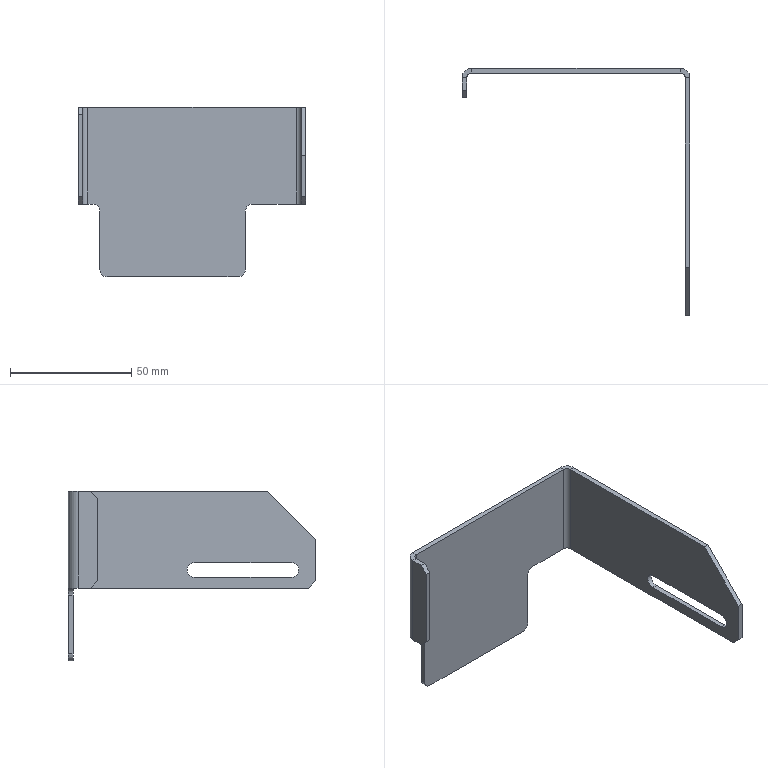Part | NX | features BREP 1 | 1 solid | 38 faces | box 94 x 102 x 70 mm | volume 18750 mm3 | plane 28 | cylinder 10 | commonest cylinder face diameters 6 x6 4 x2 8 x2
STEP:
#1=CARTESIAN_POINT('',(-43.,2.,-20.));
#2=VERTEX_POINT('',#1);
#3=CARTESIAN_POINT('',(-41.,2.,-20.));
#4=VERTEX_POINT('',#3);
#5=CARTESIAN_POINT('',(-45.,2.,-20.));
#6=DIRECTION('',(1.,0.,0.));
#7=VECTOR('',#6,1000.);
#8=LINE('',#5,#7);
#9=EDGE_CURVE('',#2,#4,#8,.T.);
#10=ORIENTED_EDGE('',*,*,#9,.T.);
#11=CARTESIAN_POINT('',(-41.,0.,-20.));
#12=VERTEX_POINT('',#11);
#13=CARTESIAN_POINT('',(-41.,-2.,-20.));
#14=DIRECTION('',(0.,-1.,0.));
#15=VECTOR('',#14,1000.);
#16=LINE('',#13,#15);
#17=EDGE_CURVE('',#4,#12,#16,.T.);
#18=ORIENTED_EDGE('',*,*,#17,.T.);
#19=CARTESIAN_POINT('',(-43.,0.,-20.));
#20=VERTEX_POINT('',#19);
#21=CARTESIAN_POINT('',(-45.,0.,-20.));
#22=DIRECTION('',(1.,0.,0.));
#23=VECTOR('',#22,1000.);
#24=LINE('',#21,#23);
#25=EDGE_CURVE('',#20,#12,#24,.T.);
#26=ORIENTED_EDGE('',*,*,#25,.F.);
#27=CARTESIAN_POINT('',(-43.,0.,-20.));
#28=DIRECTION('',(0.,1.,0.));
#29=VECTOR('',#28,1000.);
#30=LINE('',#27,#29);
#31=EDGE_CURVE('',#20,#2,#30,.T.);
#32=ORIENTED_EDGE('',*,*,#31,.T.);
#33=EDGE_LOOP('',(#10,#18,#26,#32));
#34=FACE_BOUND('',#33,.T.);
#35=CARTESIAN_POINT('',(43.,-2.,-20.));
#36=DIRECTION('',(0.,0.,1.));
#37=DIRECTION('',(-1.,0.,0.));
#38=AXIS2_PLACEMENT_3D('',#35,#36,#37);
#39=PLANE('',#38);
#40=ADVANCED_FACE('',(#34),#39,.F.);
#41=CARTESIAN_POINT('',(22.,2.,-23.));
#42=VERTEX_POINT('',#41);
#43=CARTESIAN_POINT('',(22.,2.,-47.));
#44=VERTEX_POINT('',#43);
#45=CARTESIAN_POINT('',(22.,2.,-20.));
#46=DIRECTION('',(0.,0.,-1.));
#47=VECTOR('',#46,1000.);
#48=LINE('',#45,#47);
#49=EDGE_CURVE('',#42,#44,#48,.T.);
#50=ORIENTED_EDGE('',*,*,#49,.T.);
#51=CARTESIAN_POINT('',(19.,2.,-50.));
#52=VERTEX_POINT('',#51);
#53=CARTESIAN_POINT('',(19.,2.,-47.));
#54=DIRECTION('',(0.,1.,0.));
#55=DIRECTION('',(0.,0.,1.));
#56=AXIS2_PLACEMENT_3D('',#53,#54,#55);
#57=CIRCLE('',#56,3.);
#58=EDGE_CURVE('',#44,#52,#57,.T.);
#59=ORIENTED_EDGE('',*,*,#58,.T.);
#60=CARTESIAN_POINT('',(-35.,2.,-50.));
#61=VERTEX_POINT('',#60);
#62=CARTESIAN_POINT('',(-38.,2.,-50.));
#63=DIRECTION('',(-1.,0.,0.));
#64=VECTOR('',#63,1000.);
#65=LINE('',#62,#64);
#66=EDGE_CURVE('',#52,#61,#65,.T.);
#67=ORIENTED_EDGE('',*,*,#66,.T.);
#68=CARTESIAN_POINT('',(-38.,2.,-47.));
#69=VERTEX_POINT('',#68);
#70=CARTESIAN_POINT('',(-35.,2.,-47.));
#71=DIRECTION('',(0.,1.,0.));
#72=DIRECTION('',(0.,0.,1.));
#73=AXIS2_PLACEMENT_3D('',#70,#71,#72);
#74=CIRCLE('',#73,3.);
#75=EDGE_CURVE('',#61,#69,#74,.T.);
#76=ORIENTED_EDGE('',*,*,#75,.T.);
#77=CARTESIAN_POINT('',(-38.,2.,-23.));
#78=VERTEX_POINT('',#77);
#79=CARTESIAN_POINT('',(-38.,2.,-20.));
#80=DIRECTION('',(0.,0.,1.));
#81=VECTOR('',#80,1000.);
#82=LINE('',#79,#81);
#83=EDGE_CURVE('',#69,#78,#82,.T.);
#84=ORIENTED_EDGE('',*,*,#83,.T.);
#85=CARTESIAN_POINT('',(-41.,2.,-23.));
#86=DIRECTION('',(0.,-1.,0.));
#87=DIRECTION('',(0.,0.,1.));
#88=AXIS2_PLACEMENT_3D('',#85,#86,#87);
#89=CIRCLE('',#88,3.);
#90=EDGE_CURVE('',#78,#4,#89,.T.);
#91=ORIENTED_EDGE('',*,*,#90,.T.);
#92=ORIENTED_EDGE('',*,*,#9,.F.);
#93=CARTESIAN_POINT('',(-43.,2.,20.));
#94=VERTEX_POINT('',#93);
#95=CARTESIAN_POINT('',(-43.,2.,-20.));
#96=DIRECTION('',(0.,0.,1.));
#97=VECTOR('',#96,1000.);
#98=LINE('',#95,#97);
#99=EDGE_CURVE('',#2,#94,#98,.T.);
#100=ORIENTED_EDGE('',*,*,#99,.T.);
#101=CARTESIAN_POINT('',(43.,2.,20.));
#102=VERTEX_POINT('',#101);
#103=CARTESIAN_POINT('',(-45.,2.,20.));
#104=DIRECTION('',(1.,0.,0.));
#105=VECTOR('',#104,1000.);
#106=LINE('',#103,#105);
#107=EDGE_CURVE('',#94,#102,#106,.T.);
#108=ORIENTED_EDGE('',*,*,#107,.T.);
#109=CARTESIAN_POINT('',(43.,2.,-20.));
#110=VERTEX_POINT('',#109);
#111=CARTESIAN_POINT('',(43.,2.,20.));
#112=DIRECTION('',(0.,0.,-1.));
#113=VECTOR('',#112,1000.);
#114=LINE('',#111,#113);
#115=EDGE_CURVE('',#102,#110,#114,.T.);
#116=ORIENTED_EDGE('',*,*,#115,.T.);
#117=CARTESIAN_POINT('',(25.,2.,-20.));
#118=VERTEX_POINT('',#117);
#119=CARTESIAN_POINT('',(-45.,2.,-20.));
#120=DIRECTION('',(1.,0.,0.));
#121=VECTOR('',#120,1000.);
#122=LINE('',#119,#121);
#123=EDGE_CURVE('',#118,#110,#122,.T.);
#124=ORIENTED_EDGE('',*,*,#123,.F.);
#125=CARTESIAN_POINT('',(25.,2.,-23.));
#126=DIRECTION('',(0.,-1.,0.));
#127=DIRECTION('',(0.,0.,1.));
#128=AXIS2_PLACEMENT_3D('',#125,#126,#127);
#129=CIRCLE('',#128,3.);
#130=EDGE_CURVE('',#118,#42,#129,.T.);
#131=ORIENTED_EDGE('',*,*,#130,.T.);
#132=EDGE_LOOP('',(#50,#59,#67,#76,#84,#91,#92,#100,#108,#116,#124,#131));
#133=FACE_BOUND('',#132,.T.);
#134=CARTESIAN_POINT('',(-45.,2.,20.));
#135=DIRECTION('',(0.,1.,0.));
#136=DIRECTION('',(0.,0.,-1.));
#137=AXIS2_PLACEMENT_3D('',#134,#135,#136);
#138=PLANE('',#137);
#139=ADVANCED_FACE('',(#133),#138,.T.);
#140=CARTESIAN_POINT('',(-35.,0.,-50.));
#141=VERTEX_POINT('',#140);
#142=CARTESIAN_POINT('',(19.,0.,-50.));
#143=VERTEX_POINT('',#142);
#144=CARTESIAN_POINT('',(-38.,0.,-50.));
#145=DIRECTION('',(1.,0.,0.));
#146=VECTOR('',#145,1000.);
#147=LINE('',#144,#146);
#148=EDGE_CURVE('',#141,#143,#147,.T.);
#149=ORIENTED_EDGE('',*,*,#148,.T.);
#150=CARTESIAN_POINT('',(22.,0.,-47.));
#151=VERTEX_POINT('',#150);
#152=CARTESIAN_POINT('',(19.,0.,-47.));
#153=DIRECTION('',(0.,-1.,0.));
#154=DIRECTION('',(0.,0.,1.));
#155=AXIS2_PLACEMENT_3D('',#152,#153,#154);
#156=CIRCLE('',#155,3.);
#157=EDGE_CURVE('',#143,#151,#156,.T.);
#158=ORIENTED_EDGE('',*,*,#157,.T.);
#159=CARTESIAN_POINT('',(22.,0.,-23.));
#160=VERTEX_POINT('',#159);
#161=CARTESIAN_POINT('',(22.,0.,-20.));
#162=DIRECTION('',(0.,0.,1.));
#163=VECTOR('',#162,1000.);
#164=LINE('',#161,#163);
#165=EDGE_CURVE('',#151,#160,#164,.T.);
#166=ORIENTED_EDGE('',*,*,#165,.T.);
#167=CARTESIAN_POINT('',(25.,0.,-20.));
#168=VERTEX_POINT('',#167);
#169=CARTESIAN_POINT('',(25.,0.,-23.));
#170=DIRECTION('',(0.,1.,0.));
#171=DIRECTION('',(0.,0.,1.));
#172=AXIS2_PLACEMENT_3D('',#169,#170,#171);
#173=CIRCLE('',#172,3.);
#174=EDGE_CURVE('',#160,#168,#173,.T.);
#175=ORIENTED_EDGE('',*,*,#174,.T.);
#176=CARTESIAN_POINT('',(43.,0.,-20.));
#177=VERTEX_POINT('',#176);
#178=CARTESIAN_POINT('',(-45.,0.,-20.));
#179=DIRECTION('',(1.,0.,0.));
#180=VECTOR('',#179,1000.);
#181=LINE('',#178,#180);
#182=EDGE_CURVE('',#168,#177,#181,.T.);
#183=ORIENTED_EDGE('',*,*,#182,.T.);
#184=CARTESIAN_POINT('',(43.,0.,20.));
#185=VERTEX_POINT('',#184);
#186=CARTESIAN_POINT('',(43.,0.,20.));
#187=DIRECTION('',(0.,0.,-1.));
#188=VECTOR('',#187,1000.);
#189=LINE('',#186,#188);
#190=EDGE_CURVE('',#185,#177,#189,.T.);
#191=ORIENTED_EDGE('',*,*,#190,.F.);
#192=CARTESIAN_POINT('',(-43.,0.,20.));
#193=VERTEX_POINT('',#192);
#194=CARTESIAN_POINT('',(-45.,0.,20.));
#195=DIRECTION('',(1.,0.,0.));
#196=VECTOR('',#195,1000.);
#197=LINE('',#194,#196);
#198=EDGE_CURVE('',#193,#185,#197,.T.);
#199=ORIENTED_EDGE('',*,*,#198,.F.);
#200=CARTESIAN_POINT('',(-43.,0.,-20.));
#201=DIRECTION('',(0.,0.,1.));
#202=VECTOR('',#201,1000.);
#203=LINE('',#200,#202);
#204=EDGE_CURVE('',#20,#193,#203,.T.);
#205=ORIENTED_EDGE('',*,*,#204,.F.);
#206=ORIENTED_EDGE('',*,*,#25,.T.);
#207=CARTESIAN_POINT('',(-38.,0.,-23.));
#208=VERTEX_POINT('',#207);
#209=CARTESIAN_POINT('',(-41.,0.,-23.));
#210=DIRECTION('',(0.,1.,0.));
#211=DIRECTION('',(0.,0.,1.));
#212=AXIS2_PLACEMENT_3D('',#209,#210,#211);
#213=CIRCLE('',#212,3.);
#214=EDGE_CURVE('',#12,#208,#213,.T.);
#215=ORIENTED_EDGE('',*,*,#214,.T.);
#216=CARTESIAN_POINT('',(-38.,0.,-47.));
#217=VERTEX_POINT('',#216);
#218=CARTESIAN_POINT('',(-38.,0.,-20.));
#219=DIRECTION('',(0.,0.,-1.));
#220=VECTOR('',#219,1000.);
#221=LINE('',#218,#220);
#222=EDGE_CURVE('',#208,#217,#221,.T.);
#223=ORIENTED_EDGE('',*,*,#222,.T.);
#224=CARTESIAN_POINT('',(-35.,0.,-47.));
#225=DIRECTION('',(0.,-1.,0.));
#226=DIRECTION('',(0.,0.,1.));
#227=AXIS2_PLACEMENT_3D('',#224,#225,#226);
#228=CIRCLE('',#227,3.);
#229=EDGE_CURVE('',#217,#141,#228,.T.);
#230=ORIENTED_EDGE('',*,*,#229,.T.);
#231=EDGE_LOOP('',(#149,#158,#166,#175,#183,#191,#199,#205,#206,#215,#223,#230));
#232=FACE_BOUND('',#231,.T.);
#233=CARTESIAN_POINT('',(-45.,0.,20.));
#234=DIRECTION('',(0.,1.,0.));
#235=DIRECTION('',(0.,0.,-1.));
#236=AXIS2_PLACEMENT_3D('',#233,#234,#235);
#237=PLANE('',#236);
#238=ADVANCED_FACE('',(#232),#237,.F.);
#239=ORIENTED_EDGE('',*,*,#182,.F.);
#240=CARTESIAN_POINT('',(25.,-2.,-20.));
#241=DIRECTION('',(0.,1.,0.));
#242=VECTOR('',#241,1000.);
#243=LINE('',#240,#242);
#244=EDGE_CURVE('',#168,#118,#243,.T.);
#245=ORIENTED_EDGE('',*,*,#244,.T.);
#246=ORIENTED_EDGE('',*,*,#123,.T.);
#247=CARTESIAN_POINT('',(43.,2.,-20.));
#248=DIRECTION('',(0.,-1.,0.));
#249=VECTOR('',#248,1000.);
#250=LINE('',#247,#249);
#251=EDGE_CURVE('',#110,#177,#250,.T.);
#252=ORIENTED_EDGE('',*,*,#251,.T.);
#253=EDGE_LOOP('',(#239,#245,#246,#252));
#254=FACE_BOUND('',#253,.T.);
#255=CARTESIAN_POINT('',(43.,-2.,-20.));
#256=DIRECTION('',(0.,0.,1.));
#257=DIRECTION('',(-1.,0.,0.));
#258=AXIS2_PLACEMENT_3D('',#255,#256,#257);
#259=PLANE('',#258);
#260=ADVANCED_FACE('',(#254),#259,.F.);
#261=CARTESIAN_POINT('',(43.,0.,20.));
#262=DIRECTION('',(0.,1.,0.));
#263=VECTOR('',#262,1000.);
#264=LINE('',#261,#263);
#265=EDGE_CURVE('',#185,#102,#264,.T.);
#266=ORIENTED_EDGE('',*,*,#265,.F.);
#267=CARTESIAN_POINT('',(45.,-2.,20.));
#268=VERTEX_POINT('',#267);
#269=CARTESIAN_POINT('',(43.,-2.,20.));
#270=DIRECTION('',(0.,0.,-1.));
#271=DIRECTION('',(1.,0.,0.));
#272=AXIS2_PLACEMENT_3D('',#269,#270,#271);
#273=CIRCLE('',#272,2.);
#274=EDGE_CURVE('',#185,#268,#273,.T.);
#275=ORIENTED_EDGE('',*,*,#274,.T.);
#276=CARTESIAN_POINT('',(47.,-2.,20.));
#277=VERTEX_POINT('',#276);
#278=CARTESIAN_POINT('',(47.,-2.,20.));
#279=DIRECTION('',(-1.,0.,0.));
#280=VECTOR('',#279,1000.);
#281=LINE('',#278,#280);
#282=EDGE_CURVE('',#277,#268,#281,.T.);
#283=ORIENTED_EDGE('',*,*,#282,.F.);
#284=CARTESIAN_POINT('',(43.,-2.,20.));
#285=DIRECTION('',(0.,0.,-1.));
#286=DIRECTION('',(1.,0.,0.));
#287=AXIS2_PLACEMENT_3D('',#284,#285,#286);
#288=CIRCLE('',#287,4.);
#289=EDGE_CURVE('',#102,#277,#288,.T.);
#290=ORIENTED_EDGE('',*,*,#289,.F.);
#291=EDGE_LOOP('',(#266,#275,#283,#290));
#292=FACE_BOUND('',#291,.T.);
#293=CARTESIAN_POINT('',(43.,0.,20.));
#294=DIRECTION('',(0.,0.,1.));
#295=DIRECTION('',(-1.,0.,0.));
#296=AXIS2_PLACEMENT_3D('',#293,#294,#295);
#297=PLANE('',#296);
#298=ADVANCED_FACE('',(#292),#297,.T.);
#299=CARTESIAN_POINT('',(-43.,0.,20.));
#300=DIRECTION('',(0.,1.,0.));
#301=VECTOR('',#300,1000.);
#302=LINE('',#299,#301);
#303=EDGE_CURVE('',#193,#94,#302,.T.);
#304=ORIENTED_EDGE('',*,*,#303,.F.);
#305=ORIENTED_EDGE('',*,*,#198,.T.);
#306=ORIENTED_EDGE('',*,*,#265,.T.);
#307=ORIENTED_EDGE('',*,*,#107,.F.);
#308=EDGE_LOOP('',(#304,#305,#306,#307));
#309=FACE_BOUND('',#308,.T.);
#310=CARTESIAN_POINT('',(47.,-2.,20.));
#311=DIRECTION('',(0.,0.,1.));
#312=DIRECTION('',(-1.,0.,0.));
#313=AXIS2_PLACEMENT_3D('',#310,#311,#312);
#314=PLANE('',#313);
#315=ADVANCED_FACE('',(#309),#314,.T.);
#316=CARTESIAN_POINT('',(45.,-2.,-20.));
#317=VERTEX_POINT('',#316);
#318=CARTESIAN_POINT('',(47.,-2.,-20.));
#319=VERTEX_POINT('',#318);
#320=CARTESIAN_POINT('',(45.,-2.,-20.));
#321=DIRECTION('',(1.,0.,0.));
#322=VECTOR('',#321,1000.);
#323=LINE('',#320,#322);
#324=EDGE_CURVE('',#317,#319,#323,.T.);
#325=ORIENTED_EDGE('',*,*,#324,.F.);
#326=CARTESIAN_POINT('',(43.,-2.,-20.));
#327=DIRECTION('',(0.,0.,-1.));
#328=DIRECTION('',(1.,0.,0.));
#329=AXIS2_PLACEMENT_3D('',#326,#327,#328);
#330=CIRCLE('',#329,2.);
#331=EDGE_CURVE('',#177,#317,#330,.T.);
#332=ORIENTED_EDGE('',*,*,#331,.F.);
#333=ORIENTED_EDGE('',*,*,#251,.F.);
#334=CARTESIAN_POINT('',(43.,-2.,-20.));
#335=DIRECTION('',(0.,0.,-1.));
#336=DIRECTION('',(1.,0.,0.));
#337=AXIS2_PLACEMENT_3D('',#334,#335,#336);
#338=CIRCLE('',#337,4.);
#339=EDGE_CURVE('',#110,#319,#338,.T.);
#340=ORIENTED_EDGE('',*,*,#339,.T.);
#341=EDGE_LOOP('',(#325,#332,#333,#340));
#342=FACE_BOUND('',#341,.T.);
#343=CARTESIAN_POINT('',(45.,-2.,-20.));
#344=DIRECTION('',(0.,0.,-1.));
#345=DIRECTION('',(1.,0.,0.));
#346=AXIS2_PLACEMENT_3D('',#343,#344,#345);
#347=PLANE('',#346);
#348=ADVANCED_FACE('',(#342),#347,.T.);
#349=CARTESIAN_POINT('',(47.,-97.,-20.));
#350=VERTEX_POINT('',#349);
#351=CARTESIAN_POINT('',(47.,0.,-20.));
#352=DIRECTION('',(0.,-1.,0.));
#353=VECTOR('',#352,1000.);
#354=LINE('',#351,#353);
#355=EDGE_CURVE('',#319,#350,#354,.T.);
#356=ORIENTED_EDGE('',*,*,#355,.T.);
#357=CARTESIAN_POINT('',(45.,-97.,-20.));
#358=VERTEX_POINT('',#357);
#359=CARTESIAN_POINT('',(43.,-97.,-20.));
#360=DIRECTION('',(-1.,0.,0.));
#361=VECTOR('',#360,1000.);
#362=LINE('',#359,#361);
#363=EDGE_CURVE('',#350,#358,#362,.T.);
#364=ORIENTED_EDGE('',*,*,#363,.T.);
#365=CARTESIAN_POINT('',(45.,0.,-20.));
#366=DIRECTION('',(0.,-1.,0.));
#367=VECTOR('',#366,1000.);
#368=LINE('',#365,#367);
#369=EDGE_CURVE('',#317,#358,#368,.T.);
#370=ORIENTED_EDGE('',*,*,#369,.F.);
#371=ORIENTED_EDGE('',*,*,#324,.T.);
#372=EDGE_LOOP('',(#356,#364,#370,#371));
#373=FACE_BOUND('',#372,.T.);
#374=CARTESIAN_POINT('',(43.,2.,-20.));
#375=DIRECTION('',(0.,0.,-1.));
#376=DIRECTION('',(1.,0.,0.));
#377=AXIS2_PLACEMENT_3D('',#374,#375,#376);
#378=PLANE('',#377);
#379=ADVANCED_FACE('',(#373),#378,.T.);
#380=CARTESIAN_POINT('',(45.,-50.,-15.5));
#381=VERTEX_POINT('',#380);
#382=CARTESIAN_POINT('',(45.,-90.,-15.5));
#383=VERTEX_POINT('',#382);
#384=CARTESIAN_POINT('',(45.,-50.,-15.5));
#385=DIRECTION('',(0.,-1.,0.));
#386=VECTOR('',#385,1000.);
#387=LINE('',#384,#386);
#388=EDGE_CURVE('',#381,#383,#387,.T.);
#389=ORIENTED_EDGE('',*,*,#388,.F.);
#390=CARTESIAN_POINT('',(45.,-50.,-9.5));
#391=VERTEX_POINT('',#390);
#392=CARTESIAN_POINT('',(45.,-50.,-12.5));
#393=DIRECTION('',(-1.,0.,0.));
#394=DIRECTION('',(0.,1.,0.));
#395=AXIS2_PLACEMENT_3D('',#392,#393,#394);
#396=CIRCLE('',#395,3.);
#397=EDGE_CURVE('',#391,#381,#396,.T.);
#398=ORIENTED_EDGE('',*,*,#397,.F.);
#399=CARTESIAN_POINT('',(45.,-90.,-9.5));
#400=VERTEX_POINT('',#399);
#401=CARTESIAN_POINT('',(45.,-50.,-9.5));
#402=DIRECTION('',(0.,1.,0.));
#403=VECTOR('',#402,1000.);
#404=LINE('',#401,#403);
#405=EDGE_CURVE('',#400,#391,#404,.T.);
#406=ORIENTED_EDGE('',*,*,#405,.F.);
#407=CARTESIAN_POINT('',(45.,-90.,-12.5));
#408=DIRECTION('',(-1.,0.,0.));
#409=DIRECTION('',(0.,1.,0.));
#410=AXIS2_PLACEMENT_3D('',#407,#408,#409);
#411=CIRCLE('',#410,3.);
#412=EDGE_CURVE('',#383,#400,#411,.T.);
#413=ORIENTED_EDGE('',*,*,#412,.F.);
#414=EDGE_LOOP('',(#389,#398,#406,#413));
#415=FACE_BOUND('',#414,.T.);
#416=CARTESIAN_POINT('',(45.,-100.,0.));
#417=VERTEX_POINT('',#416);
#418=CARTESIAN_POINT('',(45.,-100.,-17.));
#419=VERTEX_POINT('',#418);
#420=CARTESIAN_POINT('',(45.,-100.,20.));
#421=DIRECTION('',(0.,0.,-1.));
#422=VECTOR('',#421,1000.);
#423=LINE('',#420,#422);
#424=EDGE_CURVE('',#417,#419,#423,.T.);
#425=ORIENTED_EDGE('',*,*,#424,.F.);
#426=CARTESIAN_POINT('',(45.,-80.,20.));
#427=VERTEX_POINT('',#426);
#428=CARTESIAN_POINT('',(45.,-100.,0.));
#429=DIRECTION('',(0.,0.7071,0.7071));
#430=VECTOR('',#429,1000.);
#431=LINE('',#428,#430);
#432=EDGE_CURVE('',#417,#427,#431,.T.);
#433=ORIENTED_EDGE('',*,*,#432,.T.);
#434=CARTESIAN_POINT('',(45.,0.,20.));
#435=DIRECTION('',(0.,-1.,0.));
#436=VECTOR('',#435,1000.);
#437=LINE('',#434,#436);
#438=EDGE_CURVE('',#268,#427,#437,.T.);
#439=ORIENTED_EDGE('',*,*,#438,.F.);
#440=CARTESIAN_POINT('',(45.,-2.,20.));
#441=DIRECTION('',(0.,0.,-1.));
#442=VECTOR('',#441,1000.);
#443=LINE('',#440,#442);
#444=EDGE_CURVE('',#268,#317,#443,.T.);
#445=ORIENTED_EDGE('',*,*,#444,.T.);
#446=ORIENTED_EDGE('',*,*,#369,.T.);
#447=CARTESIAN_POINT('',(45.,-97.,-20.));
#448=DIRECTION('',(0.,-0.7071,0.7071));
#449=VECTOR('',#448,1000.);
#450=LINE('',#447,#449);
#451=EDGE_CURVE('',#358,#419,#450,.T.);
#452=ORIENTED_EDGE('',*,*,#451,.T.);
#453=EDGE_LOOP('',(#425,#433,#439,#445,#446,#452));
#454=FACE_BOUND('',#453,.T.);
#455=CARTESIAN_POINT('',(45.,0.,20.));
#456=DIRECTION('',(1.,0.,0.));
#457=DIRECTION('',(0.,-1.,0.));
#458=AXIS2_PLACEMENT_3D('',#455,#456,#457);
#459=PLANE('',#458);
#460=ADVANCED_FACE('',(#415,#454),#459,.F.);
#461=CARTESIAN_POINT('',(47.,-100.,0.));
#462=VERTEX_POINT('',#461);
#463=CARTESIAN_POINT('',(47.,-100.,-17.));
#464=VERTEX_POINT('',#463);
#465=CARTESIAN_POINT('',(47.,-100.,20.));
#466=DIRECTION('',(0.,0.,-1.));
#467=VECTOR('',#466,1000.);
#468=LINE('',#465,#467);
#469=EDGE_CURVE('',#462,#464,#468,.T.);
#470=ORIENTED_EDGE('',*,*,#469,.F.);
#471=CARTESIAN_POINT('',(47.,-100.,0.));
#472=DIRECTION('',(-1.,0.,0.));
#473=VECTOR('',#472,1000.);
#474=LINE('',#471,#473);
#475=EDGE_CURVE('',#462,#417,#474,.T.);
#476=ORIENTED_EDGE('',*,*,#475,.T.);
#477=ORIENTED_EDGE('',*,*,#424,.T.);
#478=CARTESIAN_POINT('',(47.,-100.,-17.));
#479=DIRECTION('',(1.,0.,0.));
#480=VECTOR('',#479,1000.);
#481=LINE('',#478,#480);
#482=EDGE_CURVE('',#419,#464,#481,.T.);
#483=ORIENTED_EDGE('',*,*,#482,.T.);
#484=EDGE_LOOP('',(#470,#476,#477,#483));
#485=FACE_BOUND('',#484,.T.);
#486=CARTESIAN_POINT('',(47.,-100.,20.));
#487=DIRECTION('',(0.,-1.,0.));
#488=DIRECTION('',(0.,0.,1.));
#489=AXIS2_PLACEMENT_3D('',#486,#487,#488);
#490=PLANE('',#489);
#491=ADVANCED_FACE('',(#485),#490,.T.);
#492=CARTESIAN_POINT('',(47.,-50.,-15.5));
#493=VERTEX_POINT('',#492);
#494=CARTESIAN_POINT('',(47.,-50.,-9.5));
#495=VERTEX_POINT('',#494);
#496=CARTESIAN_POINT('',(47.,-50.,-12.5));
#497=DIRECTION('',(1.,0.,0.));
#498=DIRECTION('',(0.,1.,0.));
#499=AXIS2_PLACEMENT_3D('',#496,#497,#498);
#500=CIRCLE('',#499,3.);
#501=EDGE_CURVE('',#493,#495,#500,.T.);
#502=ORIENTED_EDGE('',*,*,#501,.F.);
#503=CARTESIAN_POINT('',(47.,-90.,-15.5));
#504=VERTEX_POINT('',#503);
#505=CARTESIAN_POINT('',(47.,-50.,-15.5));
#506=DIRECTION('',(0.,1.,0.));
#507=VECTOR('',#506,1000.);
#508=LINE('',#505,#507);
#509=EDGE_CURVE('',#504,#493,#508,.T.);
#510=ORIENTED_EDGE('',*,*,#509,.F.);
#511=CARTESIAN_POINT('',(47.,-90.,-9.5));
#512=VERTEX_POINT('',#511);
#513=CARTESIAN_POINT('',(47.,-90.,-12.5));
#514=DIRECTION('',(1.,0.,0.));
#515=DIRECTION('',(0.,1.,0.));
#516=AXIS2_PLACEMENT_3D('',#513,#514,#515);
#517=CIRCLE('',#516,3.);
#518=EDGE_CURVE('',#512,#504,#517,.T.);
#519=ORIENTED_EDGE('',*,*,#518,.F.);
#520=CARTESIAN_POINT('',(47.,-50.,-9.5));
#521=DIRECTION('',(0.,-1.,0.));
#522=VECTOR('',#521,1000.);
#523=LINE('',#520,#522);
#524=EDGE_CURVE('',#495,#512,#523,.T.);
#525=ORIENTED_EDGE('',*,*,#524,.F.);
#526=EDGE_LOOP('',(#502,#510,#519,#525));
#527=FACE_BOUND('',#526,.T.);
#528=CARTESIAN_POINT('',(47.,-80.,20.));
#529=VERTEX_POINT('',#528);
#530=CARTESIAN_POINT('',(47.,0.,20.));
#531=DIRECTION('',(0.,-1.,0.));
#532=VECTOR('',#531,1000.);
#533=LINE('',#530,#532);
#534=EDGE_CURVE('',#277,#529,#533,.T.);
#535=ORIENTED_EDGE('',*,*,#534,.T.);
#536=CARTESIAN_POINT('',(47.,-40.,60.));
#537=DIRECTION('',(0.,-0.7071,-0.7071));
#538=VECTOR('',#537,1000.);
#539=LINE('',#536,#538);
#540=EDGE_CURVE('',#529,#462,#539,.T.);
#541=ORIENTED_EDGE('',*,*,#540,.T.);
#542=ORIENTED_EDGE('',*,*,#469,.T.);
#543=CARTESIAN_POINT('',(47.,-68.5,-48.5));
#544=DIRECTION('',(0.,0.7071,-0.7071));
#545=VECTOR('',#544,1000.);
#546=LINE('',#543,#545);
#547=EDGE_CURVE('',#464,#350,#546,.T.);
#548=ORIENTED_EDGE('',*,*,#547,.T.);
#549=ORIENTED_EDGE('',*,*,#355,.F.);
#550=CARTESIAN_POINT('',(47.,-2.,20.));
#551=DIRECTION('',(0.,0.,-1.));
#552=VECTOR('',#551,1000.);
#553=LINE('',#550,#552);
#554=EDGE_CURVE('',#277,#319,#553,.T.);
#555=ORIENTED_EDGE('',*,*,#554,.F.);
#556=EDGE_LOOP('',(#535,#541,#542,#548,#549,#555));
#557=FACE_BOUND('',#556,.T.);
#558=CARTESIAN_POINT('',(47.,0.,20.));
#559=DIRECTION('',(1.,0.,0.));
#560=DIRECTION('',(0.,-1.,0.));
#561=AXIS2_PLACEMENT_3D('',#558,#559,#560);
#562=PLANE('',#561);
#563=ADVANCED_FACE('',(#527,#557),#562,.T.);
#564=ORIENTED_EDGE('',*,*,#339,.F.);
#565=ORIENTED_EDGE('',*,*,#115,.F.);
#566=ORIENTED_EDGE('',*,*,#289,.T.);
#567=ORIENTED_EDGE('',*,*,#554,.T.);
#568=EDGE_LOOP('',(#564,#565,#566,#567));
#569=FACE_BOUND('',#568,.T.);
#570=CARTESIAN_POINT('',(43.,-2.,20.));
#571=DIRECTION('',(0.,0.,-1.));
#572=DIRECTION('',(1.,0.,0.));
#573=AXIS2_PLACEMENT_3D('',#570,#571,#572);
#574=CYLINDRICAL_SURFACE('',#573,4.);
#575=ADVANCED_FACE('',(#569),#574,.T.);
#576=ORIENTED_EDGE('',*,*,#331,.T.);
#577=ORIENTED_EDGE('',*,*,#444,.F.);
#578=ORIENTED_EDGE('',*,*,#274,.F.);
#579=ORIENTED_EDGE('',*,*,#190,.T.);
#580=EDGE_LOOP('',(#576,#577,#578,#579));
#581=FACE_BOUND('',#580,.T.);
#582=CARTESIAN_POINT('',(43.,-2.,20.));
#583=DIRECTION('',(0.,0.,-1.));
#584=DIRECTION('',(1.,0.,0.));
#585=AXIS2_PLACEMENT_3D('',#582,#583,#584);
#586=CYLINDRICAL_SURFACE('',#585,2.);
#587=ADVANCED_FACE('',(#581),#586,.F.);
#588=ORIENTED_EDGE('',*,*,#438,.T.);
#589=CARTESIAN_POINT('',(43.,-80.,20.));
#590=DIRECTION('',(1.,0.,0.));
#591=VECTOR('',#590,1000.);
#592=LINE('',#589,#591);
#593=EDGE_CURVE('',#427,#529,#592,.T.);
#594=ORIENTED_EDGE('',*,*,#593,.T.);
#595=ORIENTED_EDGE('',*,*,#534,.F.);
#596=ORIENTED_EDGE('',*,*,#282,.T.);
#597=EDGE_LOOP('',(#588,#594,#595,#596));
#598=FACE_BOUND('',#597,.T.);
#599=CARTESIAN_POINT('',(43.,-2.,20.));
#600=DIRECTION('',(0.,0.,1.));
#601=DIRECTION('',(-1.,0.,0.));
#602=AXIS2_PLACEMENT_3D('',#599,#600,#601);
#603=PLANE('',#602);
#604=ADVANCED_FACE('',(#598),#603,.T.);
#605=ORIENTED_EDGE('',*,*,#397,.T.);
#606=CARTESIAN_POINT('',(-1.39,-50.,-15.5));
#607=DIRECTION('',(1.,0.,0.));
#608=VECTOR('',#607,1000.);
#609=LINE('',#606,#608);
#610=EDGE_CURVE('',#381,#493,#609,.T.);
#611=ORIENTED_EDGE('',*,*,#610,.T.);
#612=ORIENTED_EDGE('',*,*,#501,.T.);
#613=CARTESIAN_POINT('',(-1.39,-50.,-9.5));
#614=DIRECTION('',(1.,0.,0.));
#615=VECTOR('',#614,1000.);
#616=LINE('',#613,#615);
#617=EDGE_CURVE('',#391,#495,#616,.T.);
#618=ORIENTED_EDGE('',*,*,#617,.F.);
#619=EDGE_LOOP('',(#605,#611,#612,#618));
#620=FACE_BOUND('',#619,.T.);
#621=CARTESIAN_POINT('',(-1.39,-50.,-12.5));
#622=DIRECTION('',(1.,0.,0.));
#623=DIRECTION('',(0.,-1.,0.));
#624=AXIS2_PLACEMENT_3D('',#621,#622,#623);
#625=CYLINDRICAL_SURFACE('',#624,3.);
#626=ADVANCED_FACE('',(#620),#625,.F.);
#627=ORIENTED_EDGE('',*,*,#388,.T.);
#628=CARTESIAN_POINT('',(-1.39,-90.,-15.5));
#629=DIRECTION('',(1.,0.,0.));
#630=VECTOR('',#629,1000.);
#631=LINE('',#628,#630);
#632=EDGE_CURVE('',#383,#504,#631,.T.);
#633=ORIENTED_EDGE('',*,*,#632,.T.);
#634=ORIENTED_EDGE('',*,*,#509,.T.);
#635=ORIENTED_EDGE('',*,*,#610,.F.);
#636=EDGE_LOOP('',(#627,#633,#634,#635));
#637=FACE_BOUND('',#636,.T.);
#638=CARTESIAN_POINT('',(-1.39,-50.,-15.5));
#639=DIRECTION('',(0.,0.,-1.));
#640=DIRECTION('',(0.,-1.,0.));
#641=AXIS2_PLACEMENT_3D('',#638,#639,#640);
#642=PLANE('',#641);
#643=ADVANCED_FACE('',(#637),#642,.F.);
#644=ORIENTED_EDGE('',*,*,#412,.T.);
#645=CARTESIAN_POINT('',(-1.39,-90.,-9.5));
#646=DIRECTION('',(1.,0.,0.));
#647=VECTOR('',#646,1000.);
#648=LINE('',#645,#647);
#649=EDGE_CURVE('',#400,#512,#648,.T.);
#650=ORIENTED_EDGE('',*,*,#649,.T.);
#651=ORIENTED_EDGE('',*,*,#518,.T.);
#652=ORIENTED_EDGE('',*,*,#632,.F.);
#653=EDGE_LOOP('',(#644,#650,#651,#652));
#654=FACE_BOUND('',#653,.T.);
#655=CARTESIAN_POINT('',(-1.39,-90.,-12.5));
#656=DIRECTION('',(1.,0.,0.));
#657=DIRECTION('',(0.,-1.,0.));
#658=AXIS2_PLACEMENT_3D('',#655,#656,#657);
#659=CYLINDRICAL_SURFACE('',#658,3.);
#660=ADVANCED_FACE('',(#654),#659,.F.);
#661=ORIENTED_EDGE('',*,*,#405,.T.);
#662=ORIENTED_EDGE('',*,*,#617,.T.);
#663=ORIENTED_EDGE('',*,*,#524,.T.);
#664=ORIENTED_EDGE('',*,*,#649,.F.);
#665=EDGE_LOOP('',(#661,#662,#663,#664));
#666=FACE_BOUND('',#665,.T.);
#667=CARTESIAN_POINT('',(-1.39,-50.,-9.5));
#668=DIRECTION('',(0.,0.,1.));
#669=DIRECTION('',(0.,1.,0.));
#670=AXIS2_PLACEMENT_3D('',#667,#668,#669);
#671=PLANE('',#670);
#672=ADVANCED_FACE('',(#666),#671,.F.);
#673=CARTESIAN_POINT('',(-45.,-2.,20.));
#674=VERTEX_POINT('',#673);
#675=CARTESIAN_POINT('',(-47.,-2.,20.));
#676=VERTEX_POINT('',#675);
#677=CARTESIAN_POINT('',(-45.,-2.,20.));
#678=DIRECTION('',(-1.,0.,0.));
#679=VECTOR('',#678,1000.);
#680=LINE('',#677,#679);
#681=EDGE_CURVE('',#674,#676,#680,.T.);
#682=ORIENTED_EDGE('',*,*,#681,.F.);
#683=CARTESIAN_POINT('',(-43.,-2.,20.));
#684=DIRECTION('',(0.,0.,1.));
#685=DIRECTION('',(-1.,0.,0.));
#686=AXIS2_PLACEMENT_3D('',#683,#684,#685);
#687=CIRCLE('',#686,2.);
#688=EDGE_CURVE('',#193,#674,#687,.T.);
#689=ORIENTED_EDGE('',*,*,#688,.F.);
#690=ORIENTED_EDGE('',*,*,#303,.T.);
#691=CARTESIAN_POINT('',(-43.,-2.,20.));
#692=DIRECTION('',(0.,0.,1.));
#693=DIRECTION('',(-1.,0.,0.));
#694=AXIS2_PLACEMENT_3D('',#691,#692,#693);
#695=CIRCLE('',#694,4.);
#696=EDGE_CURVE('',#94,#676,#695,.T.);
#697=ORIENTED_EDGE('',*,*,#696,.T.);
#698=EDGE_LOOP('',(#682,#689,#690,#697));
#699=FACE_BOUND('',#698,.T.);
#700=CARTESIAN_POINT('',(-43.,-2.,20.));
#701=DIRECTION('',(0.,0.,1.));
#702=DIRECTION('',(-1.,0.,0.));
#703=AXIS2_PLACEMENT_3D('',#700,#701,#702);
#704=PLANE('',#703);
#705=ADVANCED_FACE('',(#699),#704,.T.);
#706=CARTESIAN_POINT('',(-45.,-2.,-20.));
#707=VERTEX_POINT('',#706);
#708=CARTESIAN_POINT('',(-43.,-2.,-20.));
#709=DIRECTION('',(0.,0.,-1.));
#710=DIRECTION('',(-1.,0.,0.));
#711=AXIS2_PLACEMENT_3D('',#708,#709,#710);
#712=CIRCLE('',#711,2.);
#713=EDGE_CURVE('',#707,#20,#712,.T.);
#714=ORIENTED_EDGE('',*,*,#713,.F.);
#715=CARTESIAN_POINT('',(-47.,-2.,-20.));
#716=VERTEX_POINT('',#715);
#717=CARTESIAN_POINT('',(-45.,-2.,-20.));
#718=DIRECTION('',(-1.,0.,0.));
#719=VECTOR('',#718,1000.);
#720=LINE('',#717,#719);
#721=EDGE_CURVE('',#707,#716,#720,.T.);
#722=ORIENTED_EDGE('',*,*,#721,.T.);
#723=CARTESIAN_POINT('',(-43.,-2.,-20.));
#724=DIRECTION('',(0.,0.,-1.));
#725=DIRECTION('',(-1.,0.,0.));
#726=AXIS2_PLACEMENT_3D('',#723,#724,#725);
#727=CIRCLE('',#726,4.);
#728=EDGE_CURVE('',#716,#2,#727,.T.);
#729=ORIENTED_EDGE('',*,*,#728,.T.);
#730=ORIENTED_EDGE('',*,*,#31,.F.);
#731=EDGE_LOOP('',(#714,#722,#729,#730));
#732=FACE_BOUND('',#731,.T.);
#733=CARTESIAN_POINT('',(-43.,-2.,-20.));
#734=DIRECTION('',(0.,0.,1.));
#735=DIRECTION('',(-1.,0.,0.));
#736=AXIS2_PLACEMENT_3D('',#733,#734,#735);
#737=PLANE('',#736);
#738=ADVANCED_FACE('',(#732),#737,.F.);
#739=ORIENTED_EDGE('',*,*,#99,.F.);
#740=ORIENTED_EDGE('',*,*,#728,.F.);
#741=CARTESIAN_POINT('',(-47.,-2.,0.));
#742=DIRECTION('',(0.,0.,1.));
#743=VECTOR('',#742,1000.);
#744=LINE('',#741,#743);
#745=EDGE_CURVE('',#716,#676,#744,.T.);
#746=ORIENTED_EDGE('',*,*,#745,.T.);
#747=ORIENTED_EDGE('',*,*,#696,.F.);
#748=EDGE_LOOP('',(#739,#740,#746,#747));
#749=FACE_BOUND('',#748,.T.);
#750=CARTESIAN_POINT('',(-43.,-2.,-20.));
#751=DIRECTION('',(0.,0.,-1.));
#752=DIRECTION('',(1.,0.,0.));
#753=AXIS2_PLACEMENT_3D('',#750,#751,#752);
#754=CYLINDRICAL_SURFACE('',#753,4.);
#755=ADVANCED_FACE('',(#749),#754,.T.);
#756=ORIENTED_EDGE('',*,*,#204,.T.);
#757=ORIENTED_EDGE('',*,*,#688,.T.);
#758=CARTESIAN_POINT('',(-45.,-2.,20.));
#759=DIRECTION('',(0.,0.,-1.));
#760=VECTOR('',#759,1000.);
#761=LINE('',#758,#760);
#762=EDGE_CURVE('',#674,#707,#761,.T.);
#763=ORIENTED_EDGE('',*,*,#762,.T.);
#764=ORIENTED_EDGE('',*,*,#713,.T.);
#765=EDGE_LOOP('',(#756,#757,#763,#764));
#766=FACE_BOUND('',#765,.T.);
#767=CARTESIAN_POINT('',(-43.,-2.,-20.));
#768=DIRECTION('',(0.,0.,-1.));
#769=DIRECTION('',(1.,0.,0.));
#770=AXIS2_PLACEMENT_3D('',#767,#768,#769);
#771=CYLINDRICAL_SURFACE('',#770,2.);
#772=ADVANCED_FACE('',(#766),#771,.F.);
#773=CARTESIAN_POINT('',(-47.,-7.,20.));
#774=VERTEX_POINT('',#773);
#775=CARTESIAN_POINT('',(-47.,0.,20.));
#776=DIRECTION('',(0.,1.,0.));
#777=VECTOR('',#776,1000.);
#778=LINE('',#775,#777);
#779=EDGE_CURVE('',#774,#676,#778,.T.);
#780=ORIENTED_EDGE('',*,*,#779,.F.);
#781=CARTESIAN_POINT('',(-45.,-7.,20.));
#782=VERTEX_POINT('',#781);
#783=CARTESIAN_POINT('',(-47.,-7.,20.));
#784=DIRECTION('',(1.,0.,0.));
#785=VECTOR('',#784,1000.);
#786=LINE('',#783,#785);
#787=EDGE_CURVE('',#774,#782,#786,.T.);
#788=ORIENTED_EDGE('',*,*,#787,.T.);
#789=CARTESIAN_POINT('',(-45.,0.,20.));
#790=DIRECTION('',(0.,1.,0.));
#791=VECTOR('',#790,1000.);
#792=LINE('',#789,#791);
#793=EDGE_CURVE('',#782,#674,#792,.T.);
#794=ORIENTED_EDGE('',*,*,#793,.T.);
#795=ORIENTED_EDGE('',*,*,#681,.T.);
#796=EDGE_LOOP('',(#780,#788,#794,#795));
#797=FACE_BOUND('',#796,.T.);
#798=CARTESIAN_POINT('',(-47.,0.,20.));
#799=DIRECTION('',(0.,0.,-1.));
#800=DIRECTION('',(1.,0.,0.));
#801=AXIS2_PLACEMENT_3D('',#798,#799,#800);
#802=PLANE('',#801);
#803=ADVANCED_FACE('',(#797),#802,.F.);
#804=CARTESIAN_POINT('',(-45.,-7.,-20.));
#805=VERTEX_POINT('',#804);
#806=CARTESIAN_POINT('',(-45.,-10.,-20.));
#807=DIRECTION('',(0.,-1.,0.));
#808=VECTOR('',#807,1000.);
#809=LINE('',#806,#808);
#810=EDGE_CURVE('',#707,#805,#809,.T.);
#811=ORIENTED_EDGE('',*,*,#810,.T.);
#812=CARTESIAN_POINT('',(-47.,-7.,-20.));
#813=VERTEX_POINT('',#812);
#814=CARTESIAN_POINT('',(-47.,-7.,-20.));
#815=DIRECTION('',(-1.,0.,0.));
#816=VECTOR('',#815,1000.);
#817=LINE('',#814,#816);
#818=EDGE_CURVE('',#805,#813,#817,.T.);
#819=ORIENTED_EDGE('',*,*,#818,.T.);
#820=CARTESIAN_POINT('',(-47.,-10.,-20.));
#821=DIRECTION('',(0.,-1.,0.));
#822=VECTOR('',#821,1000.);
#823=LINE('',#820,#822);
#824=EDGE_CURVE('',#716,#813,#823,.T.);
#825=ORIENTED_EDGE('',*,*,#824,.F.);
#826=ORIENTED_EDGE('',*,*,#721,.F.);
#827=EDGE_LOOP('',(#811,#819,#825,#826));
#828=FACE_BOUND('',#827,.T.);
#829=CARTESIAN_POINT('',(-47.,-10.,-20.));
#830=DIRECTION('',(0.,0.,1.));
#831=DIRECTION('',(-1.,0.,0.));
#832=AXIS2_PLACEMENT_3D('',#829,#830,#831);
#833=PLANE('',#832);
#834=ADVANCED_FACE('',(#828),#833,.F.);
#835=ORIENTED_EDGE('',*,*,#824,.T.);
#836=CARTESIAN_POINT('',(-47.,-10.,-17.));
#837=VERTEX_POINT('',#836);
#838=CARTESIAN_POINT('',(-47.,-10.,-17.));
#839=DIRECTION('',(0.,-0.7071,0.7071));
#840=VECTOR('',#839,1000.);
#841=LINE('',#838,#840);
#842=EDGE_CURVE('',#813,#837,#841,.T.);
#843=ORIENTED_EDGE('',*,*,#842,.T.);
#844=CARTESIAN_POINT('',(-47.,-10.,17.));
#845=VERTEX_POINT('',#844);
#846=CARTESIAN_POINT('',(-47.,-10.,20.));
#847=DIRECTION('',(0.,0.,1.));
#848=VECTOR('',#847,1000.);
#849=LINE('',#846,#848);
#850=EDGE_CURVE('',#837,#845,#849,.T.);
#851=ORIENTED_EDGE('',*,*,#850,.T.);
#852=CARTESIAN_POINT('',(-47.,-7.,20.));
#853=DIRECTION('',(0.,0.7071,0.7071));
#854=VECTOR('',#853,1000.);
#855=LINE('',#852,#854);
#856=EDGE_CURVE('',#845,#774,#855,.T.);
#857=ORIENTED_EDGE('',*,*,#856,.T.);
#858=ORIENTED_EDGE('',*,*,#779,.T.);
#859=ORIENTED_EDGE('',*,*,#745,.F.);
#860=EDGE_LOOP('',(#835,#843,#851,#857,#858,#859));
#861=FACE_BOUND('',#860,.T.);
#862=CARTESIAN_POINT('',(-47.,0.,0.));
#863=DIRECTION('',(1.,0.,0.));
#864=DIRECTION('',(0.,-1.,0.));
#865=AXIS2_PLACEMENT_3D('',#862,#863,#864);
#866=PLANE('',#865);
#867=ADVANCED_FACE('',(#861),#866,.F.);
#868=CARTESIAN_POINT('',(-45.,-10.,-17.));
#869=VERTEX_POINT('',#868);
#870=CARTESIAN_POINT('',(-45.,-10.,17.));
#871=VERTEX_POINT('',#870);
#872=CARTESIAN_POINT('',(-45.,-10.,20.));
#873=DIRECTION('',(0.,0.,1.));
#874=VECTOR('',#873,1000.);
#875=LINE('',#872,#874);
#876=EDGE_CURVE('',#869,#871,#875,.T.);
#877=ORIENTED_EDGE('',*,*,#876,.F.);
#878=CARTESIAN_POINT('',(-45.,-13.5,-13.5));
#879=DIRECTION('',(0.,0.7071,-0.7071));
#880=VECTOR('',#879,1000.);
#881=LINE('',#878,#880);
#882=EDGE_CURVE('',#869,#805,#881,.T.);
#883=ORIENTED_EDGE('',*,*,#882,.T.);
#884=ORIENTED_EDGE('',*,*,#810,.F.);
#885=ORIENTED_EDGE('',*,*,#762,.F.);
#886=ORIENTED_EDGE('',*,*,#793,.F.);
#887=CARTESIAN_POINT('',(-45.,-13.5,13.5));
#888=DIRECTION('',(0.,-0.7071,-0.7071));
#889=VECTOR('',#888,1000.);
#890=LINE('',#887,#889);
#891=EDGE_CURVE('',#782,#871,#890,.T.);
#892=ORIENTED_EDGE('',*,*,#891,.T.);
#893=EDGE_LOOP('',(#877,#883,#884,#885,#886,#892));
#894=FACE_BOUND('',#893,.T.);
#895=CARTESIAN_POINT('',(-45.,0.,0.));
#896=DIRECTION('',(1.,0.,0.));
#897=DIRECTION('',(0.,-1.,0.));
#898=AXIS2_PLACEMENT_3D('',#895,#896,#897);
#899=PLANE('',#898);
#900=ADVANCED_FACE('',(#894),#899,.T.);
#901=ORIENTED_EDGE('',*,*,#850,.F.);
#902=CARTESIAN_POINT('',(-47.,-10.,-17.));
#903=DIRECTION('',(1.,0.,0.));
#904=VECTOR('',#903,1000.);
#905=LINE('',#902,#904);
#906=EDGE_CURVE('',#837,#869,#905,.T.);
#907=ORIENTED_EDGE('',*,*,#906,.T.);
#908=ORIENTED_EDGE('',*,*,#876,.T.);
#909=CARTESIAN_POINT('',(-47.,-10.,17.));
#910=DIRECTION('',(-1.,0.,0.));
#911=VECTOR('',#910,1000.);
#912=LINE('',#909,#911);
#913=EDGE_CURVE('',#871,#845,#912,.T.);
#914=ORIENTED_EDGE('',*,*,#913,.T.);
#915=EDGE_LOOP('',(#901,#907,#908,#914));
#916=FACE_BOUND('',#915,.T.);
#917=CARTESIAN_POINT('',(-47.,-10.,20.));
#918=DIRECTION('',(0.,1.,0.));
#919=DIRECTION('',(1.,0.,0.));
#920=AXIS2_PLACEMENT_3D('',#917,#918,#919);
#921=PLANE('',#920);
#922=ADVANCED_FACE('',(#916),#921,.F.);
#923=ORIENTED_EDGE('',*,*,#547,.F.);
#924=ORIENTED_EDGE('',*,*,#482,.F.);
#925=ORIENTED_EDGE('',*,*,#451,.F.);
#926=ORIENTED_EDGE('',*,*,#363,.F.);
#927=EDGE_LOOP('',(#923,#924,#925,#926));
#928=FACE_BOUND('',#927,.T.);
#929=CARTESIAN_POINT('',(43.,-97.,-20.));
#930=DIRECTION('',(0.,0.7071,0.7071));
#931=DIRECTION('',(1.,0.,0.));
#932=AXIS2_PLACEMENT_3D('',#929,#930,#931);
#933=PLANE('',#932);
#934=ADVANCED_FACE('',(#928),#933,.F.);
#935=ORIENTED_EDGE('',*,*,#842,.F.);
#936=ORIENTED_EDGE('',*,*,#818,.F.);
#937=ORIENTED_EDGE('',*,*,#882,.F.);
#938=ORIENTED_EDGE('',*,*,#906,.F.);
#939=EDGE_LOOP('',(#935,#936,#937,#938));
#940=FACE_BOUND('',#939,.T.);
#941=CARTESIAN_POINT('',(-47.,-10.,-17.));
#942=DIRECTION('',(0.,0.7071,0.7071));
#943=DIRECTION('',(-1.,0.,0.));
#944=AXIS2_PLACEMENT_3D('',#941,#942,#943);
#945=PLANE('',#944);
#946=ADVANCED_FACE('',(#940),#945,.F.);
#947=ORIENTED_EDGE('',*,*,#856,.F.);
#948=ORIENTED_EDGE('',*,*,#913,.F.);
#949=ORIENTED_EDGE('',*,*,#891,.F.);
#950=ORIENTED_EDGE('',*,*,#787,.F.);
#951=EDGE_LOOP('',(#947,#948,#949,#950));
#952=FACE_BOUND('',#951,.T.);
#953=CARTESIAN_POINT('',(-47.,-7.,20.));
#954=DIRECTION('',(0.,0.7071,-0.7071));
#955=DIRECTION('',(-1.,0.,0.));
#956=AXIS2_PLACEMENT_3D('',#953,#954,#955);
#957=PLANE('',#956);
#958=ADVANCED_FACE('',(#952),#957,.F.);
#959=ORIENTED_EDGE('',*,*,#540,.F.);
#960=ORIENTED_EDGE('',*,*,#593,.F.);
#961=ORIENTED_EDGE('',*,*,#432,.F.);
#962=ORIENTED_EDGE('',*,*,#475,.F.);
#963=EDGE_LOOP('',(#959,#960,#961,#962));
#964=FACE_BOUND('',#963,.T.);
#965=CARTESIAN_POINT('',(47.,-100.,0.));
#966=DIRECTION('',(0.,0.7071,-0.7071));
#967=DIRECTION('',(1.,0.,0.));
#968=AXIS2_PLACEMENT_3D('',#965,#966,#967);
#969=PLANE('',#968);
#970=ADVANCED_FACE('',(#964),#969,.F.);
#971=ORIENTED_EDGE('',*,*,#222,.F.);
#972=CARTESIAN_POINT('',(-38.,-67.082,-23.));
#973=DIRECTION('',(0.,1.,0.));
#974=VECTOR('',#973,1000.);
#975=LINE('',#972,#974);
#976=EDGE_CURVE('',#208,#78,#975,.T.);
#977=ORIENTED_EDGE('',*,*,#976,.T.);
#978=ORIENTED_EDGE('',*,*,#83,.F.);
#979=CARTESIAN_POINT('',(-38.,-67.082,-47.));
#980=DIRECTION('',(0.,-1.,0.));
#981=VECTOR('',#980,1000.);
#982=LINE('',#979,#981);
#983=EDGE_CURVE('',#69,#217,#982,.T.);
#984=ORIENTED_EDGE('',*,*,#983,.T.);
#985=EDGE_LOOP('',(#971,#977,#978,#984));
#986=FACE_BOUND('',#985,.T.);
#987=CARTESIAN_POINT('',(-38.,-67.082,-20.));
#988=DIRECTION('',(-1.,0.,0.));
#989=DIRECTION('',(0.,0.,-1.));
#990=AXIS2_PLACEMENT_3D('',#987,#988,#989);
#991=PLANE('',#990);
#992=ADVANCED_FACE('',(#986),#991,.T.);
#993=ORIENTED_EDGE('',*,*,#66,.F.);
#994=CARTESIAN_POINT('',(19.,-67.082,-50.));
#995=DIRECTION('',(0.,-1.,0.));
#996=VECTOR('',#995,1000.);
#997=LINE('',#994,#996);
#998=EDGE_CURVE('',#52,#143,#997,.T.);
#999=ORIENTED_EDGE('',*,*,#998,.T.);
#1000=ORIENTED_EDGE('',*,*,#148,.F.);
#1001=CARTESIAN_POINT('',(-35.,-67.082,-50.));
#1002=DIRECTION('',(0.,1.,0.));
#1003=VECTOR('',#1002,1000.);
#1004=LINE('',#1001,#1003);
#1005=EDGE_CURVE('',#141,#61,#1004,.T.);
#1006=ORIENTED_EDGE('',*,*,#1005,.T.);
#1007=EDGE_LOOP('',(#993,#999,#1000,#1006));
#1008=FACE_BOUND('',#1007,.T.);
#1009=CARTESIAN_POINT('',(-38.,-67.082,-50.));
#1010=DIRECTION('',(0.,0.,-1.));
#1011=DIRECTION('',(1.,0.,0.));
#1012=AXIS2_PLACEMENT_3D('',#1009,#1010,#1011);
#1013=PLANE('',#1012);
#1014=ADVANCED_FACE('',(#1008),#1013,.T.);
#1015=ORIENTED_EDGE('',*,*,#49,.F.);
#1016=CARTESIAN_POINT('',(22.,-67.082,-23.));
#1017=DIRECTION('',(0.,-1.,0.));
#1018=VECTOR('',#1017,1000.);
#1019=LINE('',#1016,#1018);
#1020=EDGE_CURVE('',#42,#160,#1019,.T.);
#1021=ORIENTED_EDGE('',*,*,#1020,.T.);
#1022=ORIENTED_EDGE('',*,*,#165,.F.);
#1023=CARTESIAN_POINT('',(22.,-67.082,-47.));
#1024=DIRECTION('',(0.,1.,0.));
#1025=VECTOR('',#1024,1000.);
#1026=LINE('',#1023,#1025);
#1027=EDGE_CURVE('',#151,#44,#1026,.T.);
#1028=ORIENTED_EDGE('',*,*,#1027,.T.);
#1029=EDGE_LOOP('',(#1015,#1021,#1022,#1028));
#1030=FACE_BOUND('',#1029,.T.);
#1031=CARTESIAN_POINT('',(22.,-67.082,-20.));
#1032=DIRECTION('',(1.,0.,0.));
#1033=DIRECTION('',(0.,0.,1.));
#1034=AXIS2_PLACEMENT_3D('',#1031,#1032,#1033);
#1035=PLANE('',#1034);
#1036=ADVANCED_FACE('',(#1030),#1035,.T.);
#1037=ORIENTED_EDGE('',*,*,#174,.F.);
#1038=ORIENTED_EDGE('',*,*,#1020,.F.);
#1039=ORIENTED_EDGE('',*,*,#130,.F.);
#1040=ORIENTED_EDGE('',*,*,#244,.F.);
#1041=EDGE_LOOP('',(#1037,#1038,#1039,#1040));
#1042=FACE_BOUND('',#1041,.T.);
#1043=CARTESIAN_POINT('',(25.,-2.,-23.));
#1044=DIRECTION('',(0.,1.,0.));
#1045=DIRECTION('',(0.,0.,-1.));
#1046=AXIS2_PLACEMENT_3D('',#1043,#1044,#1045);
#1047=CYLINDRICAL_SURFACE('',#1046,3.);
#1048=ADVANCED_FACE('',(#1042),#1047,.F.);
#1049=ORIENTED_EDGE('',*,*,#214,.F.);
#1050=ORIENTED_EDGE('',*,*,#17,.F.);
#1051=ORIENTED_EDGE('',*,*,#90,.F.);
#1052=ORIENTED_EDGE('',*,*,#976,.F.);
#1053=EDGE_LOOP('',(#1049,#1050,#1051,#1052));
#1054=FACE_BOUND('',#1053,.T.);
#1055=CARTESIAN_POINT('',(-41.,-67.082,-23.));
#1056=DIRECTION('',(0.,1.,0.));
#1057=DIRECTION('',(0.,0.,-1.));
#1058=AXIS2_PLACEMENT_3D('',#1055,#1056,#1057);
#1059=CYLINDRICAL_SURFACE('',#1058,3.);
#1060=ADVANCED_FACE('',(#1054),#1059,.F.);
#1061=ORIENTED_EDGE('',*,*,#157,.F.);
#1062=ORIENTED_EDGE('',*,*,#998,.F.);
#1063=ORIENTED_EDGE('',*,*,#58,.F.);
#1064=ORIENTED_EDGE('',*,*,#1027,.F.);
#1065=EDGE_LOOP('',(#1061,#1062,#1063,#1064));
#1066=FACE_BOUND('',#1065,.T.);
#1067=CARTESIAN_POINT('',(19.,-67.082,-47.));
#1068=DIRECTION('',(0.,1.,0.));
#1069=DIRECTION('',(0.,0.,-1.));
#1070=AXIS2_PLACEMENT_3D('',#1067,#1068,#1069);
#1071=CYLINDRICAL_SURFACE('',#1070,3.);
#1072=ADVANCED_FACE('',(#1066),#1071,.T.);
#1073=ORIENTED_EDGE('',*,*,#229,.F.);
#1074=ORIENTED_EDGE('',*,*,#983,.F.);
#1075=ORIENTED_EDGE('',*,*,#75,.F.);
#1076=ORIENTED_EDGE('',*,*,#1005,.F.);
#1077=EDGE_LOOP('',(#1073,#1074,#1075,#1076));
#1078=FACE_BOUND('',#1077,.T.);
#1079=CARTESIAN_POINT('',(-35.,-67.082,-47.));
#1080=DIRECTION('',(0.,1.,0.));
#1081=DIRECTION('',(0.,0.,-1.));
#1082=AXIS2_PLACEMENT_3D('',#1079,#1080,#1081);
#1083=CYLINDRICAL_SURFACE('',#1082,3.);
#1084=ADVANCED_FACE('',(#1078),#1083,.T.);
#1085=CLOSED_SHELL('',(#40,#139,#238,#260,#298,#315,#348,#379,#460,#491,#563,#575,#587,#604,#626,#643,#660,#672,#705,#738,#755,#772,#803,#834,#867,#900,#922,#934,#946,#958,#970,#992,#1014,#1036,#1048,#1060,#1072,#1084));
#1086=MANIFOLD_SOLID_BREP('',#1085);
#1087=(LENGTH_UNIT()NAMED_UNIT(*)SI_UNIT(.MILLI.,.METRE.));
#1088=UNCERTAINTY_MEASURE_WITH_UNIT(LENGTH_MEASURE(0.00001),#1087,'','');
#1089=(NAMED_UNIT(*)PLANE_ANGLE_UNIT()SI_UNIT($,.RADIAN.));
#1090=(NAMED_UNIT(*)SI_UNIT($,.STERADIAN.)SOLID_ANGLE_UNIT());
#1091=(GEOMETRIC_REPRESENTATION_CONTEXT(3)GLOBAL_UNCERTAINTY_ASSIGNED_CONTEXT((#1088))GLOBAL_UNIT_ASSIGNED_CONTEXT((#1087,#1089,#1090))REPRESENTATION_CONTEXT('',''));
#1092=ADVANCED_BREP_SHAPE_REPRESENTATION('',(#1086),#1091);